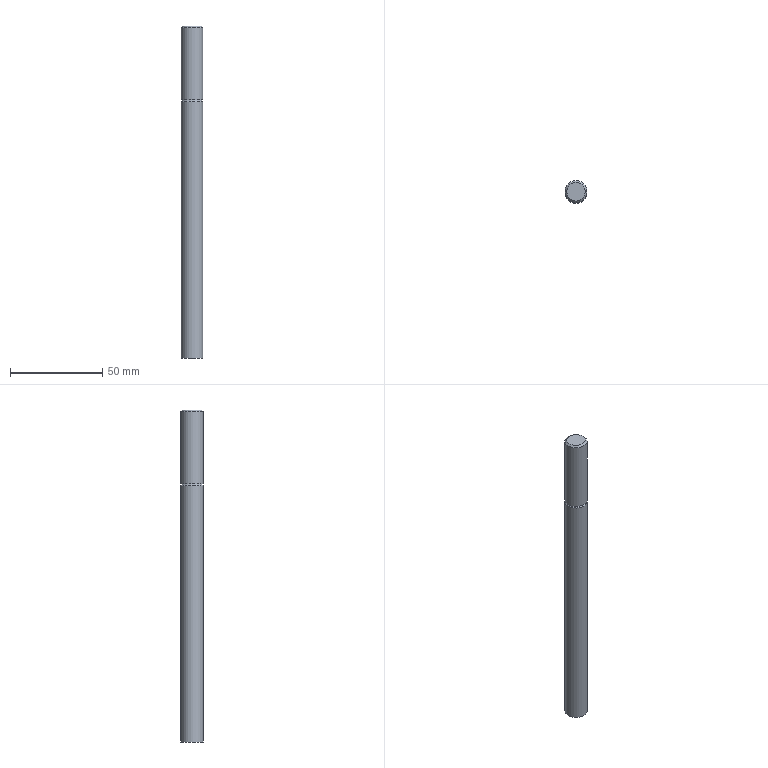Part | STEP file | tige_m12_nf_e_27_801_ecrou_h_01 | 1 solid | 7 faces | box 12 x 12 x 180 mm | volume 20325 mm3 | plane 3 | cylinder 2 | cone 2 | commonest cylinder face diameters 12 x2
STEP:
#1=CARTESIAN_POINT('',(0.,0.,0.));
#2=DIRECTION('',(0.,0.,1.));
#3=DIRECTION('',(1.,0.,0.));
#4=AXIS2_PLACEMENT_3D('',#1,#2,#3);
#5=CARTESIAN_POINT('',(0.,6.,0.));
#6=VERTEX_POINT('',#5);
#7=CARTESIAN_POINT('',(0.,0.,0.));
#8=DIRECTION('',(0.,0.,1.));
#9=DIRECTION('',(0.,1.,0.));
#10=AXIS2_PLACEMENT_3D('',#7,#8,#9);
#11=CIRCLE('',#10,6.);
#12=CARTESIAN_POINT('',(0.,3.,0.));
#13=DIRECTION('',(0.,0.,-1.));
#14=DIRECTION('',(0.,-1.,0.));
#15=AXIS2_PLACEMENT_3D('',#12,#13,#14);
#16=PLANE('',#15);
#17=CARTESIAN_POINT('',(-3.,0.));
#18=CARTESIAN_POINT('',(-3.,10.392));
#19=CARTESIAN_POINT('',(6.,5.196));
#20=CARTESIAN_POINT('',(15.,0.));
#21=CARTESIAN_POINT('',(6.,-5.196));
#22=CARTESIAN_POINT('',(-3.,-10.392));
#23=CARTESIAN_POINT('',(-3.,0.));
#24=(BOUNDED_CURVE()B_SPLINE_CURVE(2,(#17,#18,#19,#20,#21,#22,#23),.UNSPECIFIED.,.T.,.F.)B_SPLINE_CURVE_WITH_KNOTS((1,2,2,2,2,1),(-2.094,0.,2.094,4.189,6.283,8.378),.UNSPECIFIED.)CURVE()GEOMETRIC_REPRESENTATION_ITEM()RATIONAL_B_SPLINE_CURVE((1.,0.5,1.,0.5,1.,0.5,1.))REPRESENTATION_ITEM(''));
#25=(GEOMETRIC_REPRESENTATION_CONTEXT(2)PARAMETRIC_REPRESENTATION_CONTEXT()REPRESENTATION_CONTEXT('',''));
#26=DEFINITIONAL_REPRESENTATION('',(#24),#25);
#27=PCURVE('',#16,#26);
#28=CARTESIAN_POINT('',(0.,0.,69.526));
#29=DIRECTION('',(0.,0.,1.));
#30=DIRECTION('',(0.,1.,0.));
#31=AXIS2_PLACEMENT_3D('',#28,#29,#30);
#32=CYLINDRICAL_SURFACE('',#31,6.);
#33=CARTESIAN_POINT('',(0.,-69.526));
#34=DIRECTION('',(1.,0.));
#35=VECTOR('',#34,1.);
#36=LINE('',#33,#35);
#37=(GEOMETRIC_REPRESENTATION_CONTEXT(2)PARAMETRIC_REPRESENTATION_CONTEXT()REPRESENTATION_CONTEXT('',''));
#38=DEFINITIONAL_REPRESENTATION('',(#36),#37);
#39=PCURVE('',#32,#38);
#40=SURFACE_CURVE('',#11,(#27,#39),.PCURVE_S1.);
#41=EDGE_CURVE('',#6,#6,#40,.T.);
#42=ORIENTED_EDGE('',*,*,#41,.F.);
#43=EDGE_LOOP('',(#42));
#44=FACE_BOUND('',#43,.T.);
#45=ADVANCED_FACE('',(#44),#16,.T.);
#46=CARTESIAN_POINT('',(0.,6.,139.053));
#47=VERTEX_POINT('',#46);
#48=CARTESIAN_POINT('',(0.,0.,139.053));
#49=DIRECTION('',(0.,0.,1.));
#50=DIRECTION('',(0.,1.,0.));
#51=AXIS2_PLACEMENT_3D('',#48,#49,#50);
#52=CIRCLE('',#51,6.);
#53=CARTESIAN_POINT('',(0.,69.526));
#54=DIRECTION('',(1.,0.));
#55=VECTOR('',#54,1.);
#56=LINE('',#53,#55);
#57=(GEOMETRIC_REPRESENTATION_CONTEXT(2)PARAMETRIC_REPRESENTATION_CONTEXT()REPRESENTATION_CONTEXT('',''));
#58=DEFINITIONAL_REPRESENTATION('',(#56),#57);
#59=PCURVE('',#32,#58);
#60=CARTESIAN_POINT('',(0.,0.,139.526));
#61=DIRECTION('',(0.,0.,-1.));
#62=DIRECTION('',(0.,1.,0.));
#63=AXIS2_PLACEMENT_3D('',#60,#61,#62);
#64=CONICAL_SURFACE('',#63,5.526,0.7854);
#65=CARTESIAN_POINT('',(6.283,0.4736));
#66=DIRECTION('',(-1.,0.));
#67=VECTOR('',#66,1.);
#68=LINE('',#65,#67);
#69=(GEOMETRIC_REPRESENTATION_CONTEXT(2)PARAMETRIC_REPRESENTATION_CONTEXT()REPRESENTATION_CONTEXT('',''));
#70=DEFINITIONAL_REPRESENTATION('',(#68),#69);
#71=PCURVE('',#64,#70);
#72=SURFACE_CURVE('',#52,(#59,#71),.PCURVE_S1.);
#73=EDGE_CURVE('',#47,#47,#72,.T.);
#74=ORIENTED_EDGE('',*,*,#73,.F.);
#75=CARTESIAN_POINT('',(0.,6.,0.));
#76=CARTESIAN_POINT('',(0.,6.,139.053));
#77=B_SPLINE_CURVE_WITH_KNOTS('',1,(#75,#76),.UNSPECIFIED.,.F.,.F.,(2,2),(-69.526,69.526),.PIECEWISE_BEZIER_KNOTS.);
#78=CARTESIAN_POINT('',(0.,0.));
#79=DIRECTION('',(0.,1.));
#80=VECTOR('',#79,1.);
#81=LINE('',#78,#80);
#82=(GEOMETRIC_REPRESENTATION_CONTEXT(2)PARAMETRIC_REPRESENTATION_CONTEXT()REPRESENTATION_CONTEXT('',''));
#83=DEFINITIONAL_REPRESENTATION('',(#81),#82);
#84=PCURVE('',#32,#83);
#85=CARTESIAN_POINT('',(6.283,0.));
#86=DIRECTION('',(0.,1.));
#87=VECTOR('',#86,1.);
#88=LINE('',#85,#87);
#89=(GEOMETRIC_REPRESENTATION_CONTEXT(2)PARAMETRIC_REPRESENTATION_CONTEXT()REPRESENTATION_CONTEXT('',''));
#90=DEFINITIONAL_REPRESENTATION('',(#88),#89);
#91=PCURVE('',#32,#90);
#92=SEAM_CURVE('',#77,(#84,#91),.PCURVE_S1.);
#93=EDGE_CURVE('',#6,#47,#92,.T.);
#94=ORIENTED_EDGE('',*,*,#93,.F.);
#95=ORIENTED_EDGE('',*,*,#41,.T.);
#96=ORIENTED_EDGE('',*,*,#93,.T.);
#97=EDGE_LOOP('',(#74,#94,#95,#96));
#98=FACE_BOUND('',#97,.T.);
#99=ADVANCED_FACE('',(#98),#32,.T.);
#100=CARTESIAN_POINT('',(0.,5.053,140.));
#101=VERTEX_POINT('',#100);
#102=CARTESIAN_POINT('',(0.,0.,140.));
#103=DIRECTION('',(0.,0.,1.));
#104=DIRECTION('',(0.,1.,0.));
#105=AXIS2_PLACEMENT_3D('',#102,#103,#104);
#106=CIRCLE('',#105,5.053);
#107=CARTESIAN_POINT('',(6.283,-0.4736));
#108=DIRECTION('',(-1.,0.));
#109=VECTOR('',#108,1.);
#110=LINE('',#107,#109);
#111=(GEOMETRIC_REPRESENTATION_CONTEXT(2)PARAMETRIC_REPRESENTATION_CONTEXT()REPRESENTATION_CONTEXT('',''));
#112=DEFINITIONAL_REPRESENTATION('',(#110),#111);
#113=PCURVE('',#64,#112);
#114=CARTESIAN_POINT('',(0.,5.526,140.));
#115=DIRECTION('',(0.,0.,-1.));
#116=DIRECTION('',(0.,-1.,0.));
#117=AXIS2_PLACEMENT_3D('',#114,#115,#116);
#118=PLANE('',#117);
#119=CARTESIAN_POINT('',(0.4736,0.));
#120=CARTESIAN_POINT('',(0.4736,8.752));
#121=CARTESIAN_POINT('',(8.053,4.376));
#122=CARTESIAN_POINT('',(15.632,0.));
#123=CARTESIAN_POINT('',(8.053,-4.376));
#124=CARTESIAN_POINT('',(0.4736,-8.752));
#125=CARTESIAN_POINT('',(0.4736,0.));
#126=(BOUNDED_CURVE()B_SPLINE_CURVE(2,(#119,#120,#121,#122,#123,#124,#125),.UNSPECIFIED.,.T.,.F.)B_SPLINE_CURVE_WITH_KNOTS((1,2,2,2,2,1),(-2.094,0.,2.094,4.189,6.283,8.378),.UNSPECIFIED.)CURVE()GEOMETRIC_REPRESENTATION_ITEM()RATIONAL_B_SPLINE_CURVE((1.,0.5,1.,0.5,1.,0.5,1.))REPRESENTATION_ITEM(''));
#127=(GEOMETRIC_REPRESENTATION_CONTEXT(2)PARAMETRIC_REPRESENTATION_CONTEXT()REPRESENTATION_CONTEXT('',''));
#128=DEFINITIONAL_REPRESENTATION('',(#126),#127);
#129=PCURVE('',#118,#128);
#130=SURFACE_CURVE('',#106,(#113,#129),.PCURVE_S1.);
#131=EDGE_CURVE('',#101,#101,#130,.T.);
#132=ORIENTED_EDGE('',*,*,#131,.F.);
#133=CARTESIAN_POINT('',(0.,5.053,140.));
#134=CARTESIAN_POINT('',(0.,6.,139.053));
#135=B_SPLINE_CURVE_WITH_KNOTS('',1,(#133,#134),.UNSPECIFIED.,.F.,.F.,(2,2),(-0.6698,0.6698),.PIECEWISE_BEZIER_KNOTS.);
#136=CARTESIAN_POINT('',(6.283,0.));
#137=DIRECTION('',(0.,1.));
#138=VECTOR('',#137,1.);
#139=LINE('',#136,#138);
#140=(GEOMETRIC_REPRESENTATION_CONTEXT(2)PARAMETRIC_REPRESENTATION_CONTEXT()REPRESENTATION_CONTEXT('',''));
#141=DEFINITIONAL_REPRESENTATION('',(#139),#140);
#142=PCURVE('',#64,#141);
#143=CARTESIAN_POINT('',(0.,0.));
#144=DIRECTION('',(0.,1.));
#145=VECTOR('',#144,1.);
#146=LINE('',#143,#145);
#147=(GEOMETRIC_REPRESENTATION_CONTEXT(2)PARAMETRIC_REPRESENTATION_CONTEXT()REPRESENTATION_CONTEXT('',''));
#148=DEFINITIONAL_REPRESENTATION('',(#146),#147);
#149=PCURVE('',#64,#148);
#150=SEAM_CURVE('',#135,(#142,#149),.PCURVE_S1.);
#151=EDGE_CURVE('',#101,#47,#150,.T.);
#152=ORIENTED_EDGE('',*,*,#151,.T.);
#153=ORIENTED_EDGE('',*,*,#73,.T.);
#154=ORIENTED_EDGE('',*,*,#151,.F.);
#155=EDGE_LOOP('',(#132,#152,#153,#154));
#156=FACE_BOUND('',#155,.T.);
#157=ADVANCED_FACE('',(#156),#64,.T.);
#158=CARTESIAN_POINT('',(0.,6.,140.));
#159=VERTEX_POINT('',#158);
#160=CARTESIAN_POINT('',(0.,0.,140.));
#161=DIRECTION('',(0.,0.,1.));
#162=DIRECTION('',(0.,1.,0.));
#163=AXIS2_PLACEMENT_3D('',#160,#161,#162);
#164=CIRCLE('',#163,6.);
#165=CARTESIAN_POINT('',(-0.4736,0.));
#166=CARTESIAN_POINT('',(-0.4736,10.392));
#167=CARTESIAN_POINT('',(8.526,5.196));
#168=CARTESIAN_POINT('',(17.526,0.));
#169=CARTESIAN_POINT('',(8.526,-5.196));
#170=CARTESIAN_POINT('',(-0.4736,-10.392));
#171=CARTESIAN_POINT('',(-0.4736,0.));
#172=(BOUNDED_CURVE()B_SPLINE_CURVE(2,(#165,#166,#167,#168,#169,#170,#171),.UNSPECIFIED.,.T.,.F.)B_SPLINE_CURVE_WITH_KNOTS((1,2,2,2,2,1),(-2.094,0.,2.094,4.189,6.283,8.378),.UNSPECIFIED.)CURVE()GEOMETRIC_REPRESENTATION_ITEM()RATIONAL_B_SPLINE_CURVE((1.,0.5,1.,0.5,1.,0.5,1.))REPRESENTATION_ITEM(''));
#173=(GEOMETRIC_REPRESENTATION_CONTEXT(2)PARAMETRIC_REPRESENTATION_CONTEXT()REPRESENTATION_CONTEXT('',''));
#174=DEFINITIONAL_REPRESENTATION('',(#172),#173);
#175=PCURVE('',#118,#174);
#176=CARTESIAN_POINT('',(0.,0.,159.526));
#177=DIRECTION('',(0.,0.,1.));
#178=DIRECTION('',(0.,1.,0.));
#179=AXIS2_PLACEMENT_3D('',#176,#177,#178);
#180=CYLINDRICAL_SURFACE('',#179,6.);
#181=CARTESIAN_POINT('',(0.,-19.526));
#182=DIRECTION('',(1.,0.));
#183=VECTOR('',#182,1.);
#184=LINE('',#181,#183);
#185=(GEOMETRIC_REPRESENTATION_CONTEXT(2)PARAMETRIC_REPRESENTATION_CONTEXT()REPRESENTATION_CONTEXT('',''));
#186=DEFINITIONAL_REPRESENTATION('',(#184),#185);
#187=PCURVE('',#180,#186);
#188=SURFACE_CURVE('',#164,(#175,#187),.PCURVE_S1.);
#189=EDGE_CURVE('',#159,#159,#188,.T.);
#190=ORIENTED_EDGE('',*,*,#189,.F.);
#191=EDGE_LOOP('',(#190));
#192=FACE_BOUND('',#191,.T.);
#193=ORIENTED_EDGE('',*,*,#131,.T.);
#194=EDGE_LOOP('',(#193));
#195=FACE_BOUND('',#194,.T.);
#196=ADVANCED_FACE('',(#192,#195),#118,.T.);
#197=CARTESIAN_POINT('',(0.,6.,179.053));
#198=VERTEX_POINT('',#197);
#199=CARTESIAN_POINT('',(0.,0.,179.053));
#200=DIRECTION('',(0.,0.,1.));
#201=DIRECTION('',(0.,1.,0.));
#202=AXIS2_PLACEMENT_3D('',#199,#200,#201);
#203=CIRCLE('',#202,6.);
#204=CARTESIAN_POINT('',(0.,19.526));
#205=DIRECTION('',(1.,0.));
#206=VECTOR('',#205,1.);
#207=LINE('',#204,#206);
#208=(GEOMETRIC_REPRESENTATION_CONTEXT(2)PARAMETRIC_REPRESENTATION_CONTEXT()REPRESENTATION_CONTEXT('',''));
#209=DEFINITIONAL_REPRESENTATION('',(#207),#208);
#210=PCURVE('',#180,#209);
#211=CARTESIAN_POINT('',(0.,0.,179.526));
#212=DIRECTION('',(0.,0.,-1.));
#213=DIRECTION('',(0.,1.,0.));
#214=AXIS2_PLACEMENT_3D('',#211,#212,#213);
#215=CONICAL_SURFACE('',#214,5.526,0.7854);
#216=CARTESIAN_POINT('',(6.283,0.4736));
#217=DIRECTION('',(-1.,0.));
#218=VECTOR('',#217,1.);
#219=LINE('',#216,#218);
#220=(GEOMETRIC_REPRESENTATION_CONTEXT(2)PARAMETRIC_REPRESENTATION_CONTEXT()REPRESENTATION_CONTEXT('',''));
#221=DEFINITIONAL_REPRESENTATION('',(#219),#220);
#222=PCURVE('',#215,#221);
#223=SURFACE_CURVE('',#203,(#210,#222),.PCURVE_S1.);
#224=EDGE_CURVE('',#198,#198,#223,.T.);
#225=ORIENTED_EDGE('',*,*,#224,.F.);
#226=CARTESIAN_POINT('',(0.,6.,140.));
#227=CARTESIAN_POINT('',(0.,6.,179.053));
#228=B_SPLINE_CURVE_WITH_KNOTS('',1,(#226,#227),.UNSPECIFIED.,.F.,.F.,(2,2),(-19.526,19.526),.PIECEWISE_BEZIER_KNOTS.);
#229=CARTESIAN_POINT('',(0.,0.));
#230=DIRECTION('',(0.,1.));
#231=VECTOR('',#230,1.);
#232=LINE('',#229,#231);
#233=(GEOMETRIC_REPRESENTATION_CONTEXT(2)PARAMETRIC_REPRESENTATION_CONTEXT()REPRESENTATION_CONTEXT('',''));
#234=DEFINITIONAL_REPRESENTATION('',(#232),#233);
#235=PCURVE('',#180,#234);
#236=CARTESIAN_POINT('',(6.283,0.));
#237=DIRECTION('',(0.,1.));
#238=VECTOR('',#237,1.);
#239=LINE('',#236,#238);
#240=(GEOMETRIC_REPRESENTATION_CONTEXT(2)PARAMETRIC_REPRESENTATION_CONTEXT()REPRESENTATION_CONTEXT('',''));
#241=DEFINITIONAL_REPRESENTATION('',(#239),#240);
#242=PCURVE('',#180,#241);
#243=SEAM_CURVE('',#228,(#235,#242),.PCURVE_S1.);
#244=EDGE_CURVE('',#159,#198,#243,.T.);
#245=ORIENTED_EDGE('',*,*,#244,.F.);
#246=ORIENTED_EDGE('',*,*,#189,.T.);
#247=ORIENTED_EDGE('',*,*,#244,.T.);
#248=EDGE_LOOP('',(#225,#245,#246,#247));
#249=FACE_BOUND('',#248,.T.);
#250=ADVANCED_FACE('',(#249),#180,.T.);
#251=CARTESIAN_POINT('',(0.,5.053,180.));
#252=VERTEX_POINT('',#251);
#253=CARTESIAN_POINT('',(0.,0.,180.));
#254=DIRECTION('',(0.,0.,1.));
#255=DIRECTION('',(0.,1.,0.));
#256=AXIS2_PLACEMENT_3D('',#253,#254,#255);
#257=CIRCLE('',#256,5.053);
#258=CARTESIAN_POINT('',(6.283,-0.4736));
#259=DIRECTION('',(-1.,0.));
#260=VECTOR('',#259,1.);
#261=LINE('',#258,#260);
#262=(GEOMETRIC_REPRESENTATION_CONTEXT(2)PARAMETRIC_REPRESENTATION_CONTEXT()REPRESENTATION_CONTEXT('',''));
#263=DEFINITIONAL_REPRESENTATION('',(#261),#262);
#264=PCURVE('',#215,#263);
#265=CARTESIAN_POINT('',(0.,2.526,180.));
#266=DIRECTION('',(0.,0.,1.));
#267=DIRECTION('',(0.,1.,0.));
#268=AXIS2_PLACEMENT_3D('',#265,#266,#267);
#269=PLANE('',#268);
#270=CARTESIAN_POINT('',(-2.526,0.));
#271=DIRECTION('',(1.,0.));
#272=AXIS2_PLACEMENT_2D('',#270,#271);
#273=CIRCLE('',#272,5.053);
#274=(GEOMETRIC_REPRESENTATION_CONTEXT(2)PARAMETRIC_REPRESENTATION_CONTEXT()REPRESENTATION_CONTEXT('',''));
#275=DEFINITIONAL_REPRESENTATION('',(#273),#274);
#276=PCURVE('',#269,#275);
#277=SURFACE_CURVE('',#257,(#264,#276),.PCURVE_S1.);
#278=EDGE_CURVE('',#252,#252,#277,.T.);
#279=ORIENTED_EDGE('',*,*,#278,.F.);
#280=CARTESIAN_POINT('',(0.,5.053,180.));
#281=CARTESIAN_POINT('',(0.,6.,179.053));
#282=B_SPLINE_CURVE_WITH_KNOTS('',1,(#280,#281),.UNSPECIFIED.,.F.,.F.,(2,2),(-0.6698,0.6698),.PIECEWISE_BEZIER_KNOTS.);
#283=CARTESIAN_POINT('',(6.283,0.));
#284=DIRECTION('',(0.,1.));
#285=VECTOR('',#284,1.);
#286=LINE('',#283,#285);
#287=(GEOMETRIC_REPRESENTATION_CONTEXT(2)PARAMETRIC_REPRESENTATION_CONTEXT()REPRESENTATION_CONTEXT('',''));
#288=DEFINITIONAL_REPRESENTATION('',(#286),#287);
#289=PCURVE('',#215,#288);
#290=CARTESIAN_POINT('',(0.,0.));
#291=DIRECTION('',(0.,1.));
#292=VECTOR('',#291,1.);
#293=LINE('',#290,#292);
#294=(GEOMETRIC_REPRESENTATION_CONTEXT(2)PARAMETRIC_REPRESENTATION_CONTEXT()REPRESENTATION_CONTEXT('',''));
#295=DEFINITIONAL_REPRESENTATION('',(#293),#294);
#296=PCURVE('',#215,#295);
#297=SEAM_CURVE('',#282,(#289,#296),.PCURVE_S1.);
#298=EDGE_CURVE('',#252,#198,#297,.T.);
#299=ORIENTED_EDGE('',*,*,#298,.T.);
#300=ORIENTED_EDGE('',*,*,#224,.T.);
#301=ORIENTED_EDGE('',*,*,#298,.F.);
#302=EDGE_LOOP('',(#279,#299,#300,#301));
#303=FACE_BOUND('',#302,.T.);
#304=ADVANCED_FACE('',(#303),#215,.T.);
#305=ORIENTED_EDGE('',*,*,#278,.T.);
#306=EDGE_LOOP('',(#305));
#307=FACE_BOUND('',#306,.T.);
#308=ADVANCED_FACE('',(#307),#269,.T.);
#309=CLOSED_SHELL('',(#45,#99,#157,#196,#250,#304,#308));
#310=MANIFOLD_SOLID_BREP('',#309);
#311=(LENGTH_UNIT()NAMED_UNIT(*)SI_UNIT(.MILLI.,.METRE.));
#312=UNCERTAINTY_MEASURE_WITH_UNIT(LENGTH_MEASURE(0.00001),#311,'','');
#313=(NAMED_UNIT(*)PLANE_ANGLE_UNIT()SI_UNIT($,.RADIAN.));
#314=(NAMED_UNIT(*)SI_UNIT($,.STERADIAN.)SOLID_ANGLE_UNIT());
#315=(GEOMETRIC_REPRESENTATION_CONTEXT(3)GLOBAL_UNCERTAINTY_ASSIGNED_CONTEXT((#312))GLOBAL_UNIT_ASSIGNED_CONTEXT((#311,#313,#314))REPRESENTATION_CONTEXT('',''));
#316=ADVANCED_BREP_SHAPE_REPRESENTATION('',(#4,#310),#315);